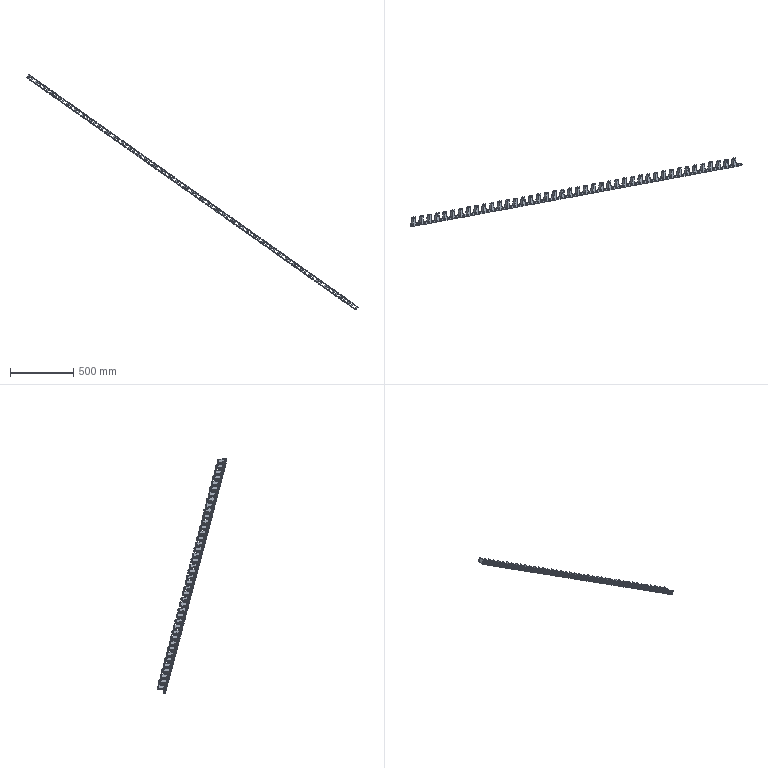Part | STEP file | left cane-feed mechanism single-link chain | 84 solids | 2184 faces | box 2616 x 545.862 x 1858 mm | volume 812261 mm3 | plane 1176 | cylinder 1008 | commonest cylinder face diameters 6 x336 18 x336 20 x126 4 x84 12 x84 16 x42